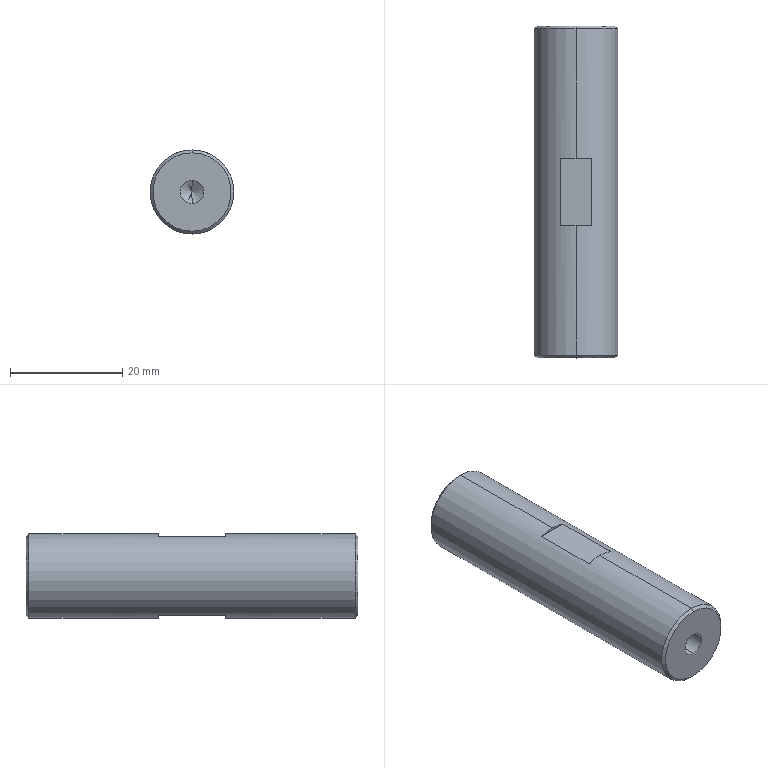Part | STEP file | ND25021-01-JDKM-72-TL | 1 solid | 22 faces | box 15 x 59.2 x 15 mm | volume 10051 mm3 | cone 8 | plane 8 | cylinder 6 | commonest cylinder face diameters 4.2 x4 15 x2
STEP:
#1=CARTESIAN_POINT('',(0.,0.,0.));
#2=DIRECTION('',(0.,0.,1.));
#3=DIRECTION('',(1.,0.,0.));
#4=AXIS2_PLACEMENT_3D('',#1,#2,#3);
#5=CARTESIAN_POINT('',(0.,29.6,7.));
#6=VERTEX_POINT('',#5);
#7=CARTESIAN_POINT('',(0.,29.6,-7.));
#8=VERTEX_POINT('',#7);
#9=CARTESIAN_POINT('',(0.,29.6,0.));
#10=DIRECTION('',(0.,1.,0.));
#11=DIRECTION('',(0.,0.,1.));
#12=AXIS2_PLACEMENT_3D('',#9,#10,#11);
#13=CIRCLE('',#12,7.);
#14=CARTESIAN_POINT('',(0.,29.6,0.));
#15=DIRECTION('',(0.,-1.,0.));
#16=DIRECTION('',(0.,0.,-1.));
#17=AXIS2_PLACEMENT_3D('',#14,#15,#16);
#18=CONICAL_SURFACE('',#17,7.,0.7854);
#19=CARTESIAN_POINT('',(3.142,0.));
#20=DIRECTION('',(-1.,0.));
#21=VECTOR('',#20,1.);
#22=LINE('',#19,#21);
#23=(GEOMETRIC_REPRESENTATION_CONTEXT(2)PARAMETRIC_REPRESENTATION_CONTEXT()REPRESENTATION_CONTEXT('',''));
#24=DEFINITIONAL_REPRESENTATION('',(#22),#23);
#25=PCURVE('',#18,#24);
#26=CARTESIAN_POINT('',(0.,29.6,0.));
#27=DIRECTION('',(0.,1.,0.));
#28=DIRECTION('',(0.,0.,1.));
#29=AXIS2_PLACEMENT_3D('',#26,#27,#28);
#30=PLANE('',#29);
#31=CARTESIAN_POINT('',(0.,0.));
#32=DIRECTION('',(1.,0.));
#33=AXIS2_PLACEMENT_2D('',#31,#32);
#34=CIRCLE('',#33,7.);
#35=(GEOMETRIC_REPRESENTATION_CONTEXT(2)PARAMETRIC_REPRESENTATION_CONTEXT()REPRESENTATION_CONTEXT('',''));
#36=DEFINITIONAL_REPRESENTATION('',(#34),#35);
#37=PCURVE('',#30,#36);
#38=SURFACE_CURVE('',#13,(#25,#37),.PCURVE_S1.);
#39=EDGE_CURVE('',#6,#8,#38,.T.);
#40=ORIENTED_EDGE('',*,*,#39,.F.);
#41=CARTESIAN_POINT('',(0.,29.1,7.5));
#42=VERTEX_POINT('',#41);
#43=CARTESIAN_POINT('',(0.,29.6,7.));
#44=DIRECTION('',(0.,-0.7071,0.7071));
#45=VECTOR('',#44,1.);
#46=LINE('',#43,#45);
#47=CARTESIAN_POINT('',(3.142,0.));
#48=DIRECTION('',(0.,1.));
#49=VECTOR('',#48,1.);
#50=LINE('',#47,#49);
#51=(GEOMETRIC_REPRESENTATION_CONTEXT(2)PARAMETRIC_REPRESENTATION_CONTEXT()REPRESENTATION_CONTEXT('',''));
#52=DEFINITIONAL_REPRESENTATION('',(#50),#51);
#53=PCURVE('',#18,#52);
#54=CARTESIAN_POINT('',(0.,29.6,0.));
#55=DIRECTION('',(0.,-1.,0.));
#56=DIRECTION('',(0.,0.,-1.));
#57=AXIS2_PLACEMENT_3D('',#54,#55,#56);
#58=CONICAL_SURFACE('',#57,7.,0.7854);
#59=CARTESIAN_POINT('',(3.142,0.));
#60=DIRECTION('',(0.,1.));
#61=VECTOR('',#60,1.);
#62=LINE('',#59,#61);
#63=(GEOMETRIC_REPRESENTATION_CONTEXT(2)PARAMETRIC_REPRESENTATION_CONTEXT()REPRESENTATION_CONTEXT('',''));
#64=DEFINITIONAL_REPRESENTATION('',(#62),#63);
#65=PCURVE('',#58,#64);
#66=SURFACE_CURVE('',#46,(#53,#65),.PCURVE_S1.);
#67=EDGE_CURVE('',#6,#42,#66,.T.);
#68=ORIENTED_EDGE('',*,*,#67,.T.);
#69=CARTESIAN_POINT('',(0.,29.1,-7.5));
#70=VERTEX_POINT('',#69);
#71=CARTESIAN_POINT('',(0.,29.1,0.));
#72=DIRECTION('',(0.,-1.,0.));
#73=DIRECTION('',(0.,0.,1.));
#74=AXIS2_PLACEMENT_3D('',#71,#72,#73);
#75=CIRCLE('',#74,7.5);
#76=CARTESIAN_POINT('',(-3.142,0.5));
#77=DIRECTION('',(1.,0.));
#78=VECTOR('',#77,1.);
#79=LINE('',#76,#78);
#80=(GEOMETRIC_REPRESENTATION_CONTEXT(2)PARAMETRIC_REPRESENTATION_CONTEXT()REPRESENTATION_CONTEXT('',''));
#81=DEFINITIONAL_REPRESENTATION('',(#79),#80);
#82=PCURVE('',#18,#81);
#83=CARTESIAN_POINT('',(0.,29.6,0.));
#84=DIRECTION('',(0.,-1.,0.));
#85=DIRECTION('',(0.,0.,-1.));
#86=AXIS2_PLACEMENT_3D('',#83,#84,#85);
#87=CYLINDRICAL_SURFACE('',#86,7.5);
#88=CARTESIAN_POINT('',(-3.142,0.5));
#89=DIRECTION('',(1.,0.));
#90=VECTOR('',#89,1.);
#91=LINE('',#88,#90);
#92=(GEOMETRIC_REPRESENTATION_CONTEXT(2)PARAMETRIC_REPRESENTATION_CONTEXT()REPRESENTATION_CONTEXT('',''));
#93=DEFINITIONAL_REPRESENTATION('',(#91),#92);
#94=PCURVE('',#87,#93);
#95=SURFACE_CURVE('',#75,(#82,#94),.PCURVE_S1.);
#96=EDGE_CURVE('',#70,#42,#95,.T.);
#97=ORIENTED_EDGE('',*,*,#96,.F.);
#98=CARTESIAN_POINT('',(0.,29.6,-7.));
#99=DIRECTION('',(0.,-0.7071,-0.7071));
#100=VECTOR('',#99,1.);
#101=LINE('',#98,#100);
#102=CARTESIAN_POINT('',(0.,0.));
#103=DIRECTION('',(0.,1.));
#104=VECTOR('',#103,1.);
#105=LINE('',#102,#104);
#106=(GEOMETRIC_REPRESENTATION_CONTEXT(2)PARAMETRIC_REPRESENTATION_CONTEXT()REPRESENTATION_CONTEXT('',''));
#107=DEFINITIONAL_REPRESENTATION('',(#105),#106);
#108=PCURVE('',#18,#107);
#109=CARTESIAN_POINT('',(6.283,0.));
#110=DIRECTION('',(0.,1.));
#111=VECTOR('',#110,1.);
#112=LINE('',#109,#111);
#113=(GEOMETRIC_REPRESENTATION_CONTEXT(2)PARAMETRIC_REPRESENTATION_CONTEXT()REPRESENTATION_CONTEXT('',''));
#114=DEFINITIONAL_REPRESENTATION('',(#112),#113);
#115=PCURVE('',#58,#114);
#116=SURFACE_CURVE('',#101,(#108,#115),.PCURVE_S1.);
#117=EDGE_CURVE('',#8,#70,#116,.T.);
#118=ORIENTED_EDGE('',*,*,#117,.F.);
#119=EDGE_LOOP('',(#40,#68,#97,#118));
#120=FACE_BOUND('',#119,.T.);
#121=ADVANCED_FACE('',(#120),#18,.T.);
#122=CARTESIAN_POINT('',(0.,-29.6,-7.));
#123=VERTEX_POINT('',#122);
#124=CARTESIAN_POINT('',(0.,-29.6,7.));
#125=VERTEX_POINT('',#124);
#126=CARTESIAN_POINT('',(0.,-29.6,0.));
#127=DIRECTION('',(0.,-1.,0.));
#128=DIRECTION('',(0.,0.,1.));
#129=AXIS2_PLACEMENT_3D('',#126,#127,#128);
#130=CIRCLE('',#129,7.);
#131=CARTESIAN_POINT('',(0.,-29.1,0.));
#132=DIRECTION('',(0.,1.,0.));
#133=DIRECTION('',(0.,0.,1.));
#134=AXIS2_PLACEMENT_3D('',#131,#132,#133);
#135=CONICAL_SURFACE('',#134,7.5,0.7854);
#136=CARTESIAN_POINT('',(6.283,-0.5));
#137=DIRECTION('',(-1.,0.));
#138=VECTOR('',#137,1.);
#139=LINE('',#136,#138);
#140=(GEOMETRIC_REPRESENTATION_CONTEXT(2)PARAMETRIC_REPRESENTATION_CONTEXT()REPRESENTATION_CONTEXT('',''));
#141=DEFINITIONAL_REPRESENTATION('',(#139),#140);
#142=PCURVE('',#135,#141);
#143=CARTESIAN_POINT('',(0.,-29.6,0.));
#144=DIRECTION('',(0.,1.,0.));
#145=DIRECTION('',(0.,0.,1.));
#146=AXIS2_PLACEMENT_3D('',#143,#144,#145);
#147=PLANE('',#146);
#148=CARTESIAN_POINT('',(7.,0.));
#149=CARTESIAN_POINT('',(7.,-12.124));
#150=CARTESIAN_POINT('',(-3.5,-6.062));
#151=CARTESIAN_POINT('',(-14.,0.));
#152=CARTESIAN_POINT('',(-3.5,6.062));
#153=CARTESIAN_POINT('',(7.,12.124));
#154=CARTESIAN_POINT('',(7.,0.));
#155=(BOUNDED_CURVE()B_SPLINE_CURVE(2,(#148,#149,#150,#151,#152,#153,#154),.UNSPECIFIED.,.T.,.F.)B_SPLINE_CURVE_WITH_KNOTS((1,2,2,2,2,1),(-2.094,0.,2.094,4.189,6.283,8.378),.UNSPECIFIED.)CURVE()GEOMETRIC_REPRESENTATION_ITEM()RATIONAL_B_SPLINE_CURVE((1.,0.5,1.,0.5,1.,0.5,1.))REPRESENTATION_ITEM(''));
#156=(GEOMETRIC_REPRESENTATION_CONTEXT(2)PARAMETRIC_REPRESENTATION_CONTEXT()REPRESENTATION_CONTEXT('',''));
#157=DEFINITIONAL_REPRESENTATION('',(#155),#156);
#158=PCURVE('',#147,#157);
#159=SURFACE_CURVE('',#130,(#142,#158),.PCURVE_S1.);
#160=EDGE_CURVE('',#123,#125,#159,.T.);
#161=ORIENTED_EDGE('',*,*,#160,.F.);
#162=CARTESIAN_POINT('',(0.,-29.1,-7.5));
#163=VERTEX_POINT('',#162);
#164=CARTESIAN_POINT('',(0.,-29.1,-7.5));
#165=DIRECTION('',(0.,0.7071,-0.7071));
#166=VECTOR('',#165,1.);
#167=LINE('',#164,#166);
#168=CARTESIAN_POINT('',(3.142,0.));
#169=DIRECTION('',(0.,1.));
#170=VECTOR('',#169,1.);
#171=LINE('',#168,#170);
#172=(GEOMETRIC_REPRESENTATION_CONTEXT(2)PARAMETRIC_REPRESENTATION_CONTEXT()REPRESENTATION_CONTEXT('',''));
#173=DEFINITIONAL_REPRESENTATION('',(#171),#172);
#174=PCURVE('',#135,#173);
#175=CARTESIAN_POINT('',(0.,-29.1,0.));
#176=DIRECTION('',(0.,1.,0.));
#177=DIRECTION('',(0.,0.,1.));
#178=AXIS2_PLACEMENT_3D('',#175,#176,#177);
#179=CONICAL_SURFACE('',#178,7.5,0.7854);
#180=CARTESIAN_POINT('',(3.142,0.));
#181=DIRECTION('',(0.,1.));
#182=VECTOR('',#181,1.);
#183=LINE('',#180,#182);
#184=(GEOMETRIC_REPRESENTATION_CONTEXT(2)PARAMETRIC_REPRESENTATION_CONTEXT()REPRESENTATION_CONTEXT('',''));
#185=DEFINITIONAL_REPRESENTATION('',(#183),#184);
#186=PCURVE('',#179,#185);
#187=SURFACE_CURVE('',#167,(#174,#186),.PCURVE_S1.);
#188=EDGE_CURVE('',#123,#163,#187,.T.);
#189=ORIENTED_EDGE('',*,*,#188,.T.);
#190=CARTESIAN_POINT('',(0.,-29.1,7.5));
#191=VERTEX_POINT('',#190);
#192=CARTESIAN_POINT('',(0.,-29.1,0.));
#193=DIRECTION('',(0.,1.,0.));
#194=DIRECTION('',(0.,0.,1.));
#195=AXIS2_PLACEMENT_3D('',#192,#193,#194);
#196=CIRCLE('',#195,7.5);
#197=CARTESIAN_POINT('',(0.,0.));
#198=DIRECTION('',(1.,0.));
#199=VECTOR('',#198,1.);
#200=LINE('',#197,#199);
#201=(GEOMETRIC_REPRESENTATION_CONTEXT(2)PARAMETRIC_REPRESENTATION_CONTEXT()REPRESENTATION_CONTEXT('',''));
#202=DEFINITIONAL_REPRESENTATION('',(#200),#201);
#203=PCURVE('',#135,#202);
#204=CARTESIAN_POINT('',(3.142,58.7));
#205=DIRECTION('',(-1.,0.));
#206=VECTOR('',#205,1.);
#207=LINE('',#204,#206);
#208=(GEOMETRIC_REPRESENTATION_CONTEXT(2)PARAMETRIC_REPRESENTATION_CONTEXT()REPRESENTATION_CONTEXT('',''));
#209=DEFINITIONAL_REPRESENTATION('',(#207),#208);
#210=PCURVE('',#87,#209);
#211=SURFACE_CURVE('',#196,(#203,#210),.PCURVE_S1.);
#212=EDGE_CURVE('',#191,#163,#211,.T.);
#213=ORIENTED_EDGE('',*,*,#212,.F.);
#214=CARTESIAN_POINT('',(0.,-29.1,7.5));
#215=DIRECTION('',(0.,0.7071,0.7071));
#216=VECTOR('',#215,1.);
#217=LINE('',#214,#216);
#218=CARTESIAN_POINT('',(0.,0.));
#219=DIRECTION('',(0.,1.));
#220=VECTOR('',#219,1.);
#221=LINE('',#218,#220);
#222=(GEOMETRIC_REPRESENTATION_CONTEXT(2)PARAMETRIC_REPRESENTATION_CONTEXT()REPRESENTATION_CONTEXT('',''));
#223=DEFINITIONAL_REPRESENTATION('',(#221),#222);
#224=PCURVE('',#135,#223);
#225=CARTESIAN_POINT('',(6.283,0.));
#226=DIRECTION('',(0.,1.));
#227=VECTOR('',#226,1.);
#228=LINE('',#225,#227);
#229=(GEOMETRIC_REPRESENTATION_CONTEXT(2)PARAMETRIC_REPRESENTATION_CONTEXT()REPRESENTATION_CONTEXT('',''));
#230=DEFINITIONAL_REPRESENTATION('',(#228),#229);
#231=PCURVE('',#179,#230);
#232=SURFACE_CURVE('',#217,(#224,#231),.PCURVE_S1.);
#233=EDGE_CURVE('',#125,#191,#232,.T.);
#234=ORIENTED_EDGE('',*,*,#233,.F.);
#235=EDGE_LOOP('',(#161,#189,#213,#234));
#236=FACE_BOUND('',#235,.T.);
#237=ADVANCED_FACE('',(#236),#135,.T.);
#238=CARTESIAN_POINT('',(0.,-17.2,-2.1));
#239=VERTEX_POINT('',#238);
#240=CARTESIAN_POINT('',(0.,-29.6,-2.1));
#241=VERTEX_POINT('',#240);
#242=CARTESIAN_POINT('',(0.,-29.6,-2.1));
#243=DIRECTION('',(0.,-1.,0.));
#244=VECTOR('',#243,1.);
#245=LINE('',#242,#244);
#246=CARTESIAN_POINT('',(0.,-29.6,0.));
#247=DIRECTION('',(0.,-1.,0.));
#248=DIRECTION('',(0.,0.,-1.));
#249=AXIS2_PLACEMENT_3D('',#246,#247,#248);
#250=CYLINDRICAL_SURFACE('',#249,2.1);
#251=CARTESIAN_POINT('',(6.283,0.));
#252=DIRECTION('',(0.,1.));
#253=VECTOR('',#252,1.);
#254=LINE('',#251,#253);
#255=(GEOMETRIC_REPRESENTATION_CONTEXT(2)PARAMETRIC_REPRESENTATION_CONTEXT()REPRESENTATION_CONTEXT('',''));
#256=DEFINITIONAL_REPRESENTATION('',(#254),#255);
#257=PCURVE('',#250,#256);
#258=CARTESIAN_POINT('',(0.,-29.6,0.));
#259=DIRECTION('',(0.,-1.,0.));
#260=DIRECTION('',(0.,0.,-1.));
#261=AXIS2_PLACEMENT_3D('',#258,#259,#260);
#262=CYLINDRICAL_SURFACE('',#261,2.1);
#263=CARTESIAN_POINT('',(0.,0.));
#264=DIRECTION('',(0.,1.));
#265=VECTOR('',#264,1.);
#266=LINE('',#263,#265);
#267=(GEOMETRIC_REPRESENTATION_CONTEXT(2)PARAMETRIC_REPRESENTATION_CONTEXT()REPRESENTATION_CONTEXT('',''));
#268=DEFINITIONAL_REPRESENTATION('',(#266),#267);
#269=PCURVE('',#262,#268);
#270=SURFACE_CURVE('',#245,(#257,#269),.PCURVE_S1.);
#271=EDGE_CURVE('',#239,#241,#270,.T.);
#272=ORIENTED_EDGE('',*,*,#271,.T.);
#273=CARTESIAN_POINT('',(0.,-29.6,2.1));
#274=VERTEX_POINT('',#273);
#275=CARTESIAN_POINT('',(0.,-29.6,0.));
#276=DIRECTION('',(0.,-1.,0.));
#277=DIRECTION('',(0.,0.,-1.));
#278=AXIS2_PLACEMENT_3D('',#275,#276,#277);
#279=CIRCLE('',#278,2.1);
#280=CARTESIAN_POINT('',(0.,0.));
#281=DIRECTION('',(1.,0.));
#282=VECTOR('',#281,1.);
#283=LINE('',#280,#282);
#284=(GEOMETRIC_REPRESENTATION_CONTEXT(2)PARAMETRIC_REPRESENTATION_CONTEXT()REPRESENTATION_CONTEXT('',''));
#285=DEFINITIONAL_REPRESENTATION('',(#283),#284);
#286=PCURVE('',#250,#285);
#287=CARTESIAN_POINT('',(-2.1,0.));
#288=CARTESIAN_POINT('',(-2.1,3.637));
#289=CARTESIAN_POINT('',(1.05,1.819));
#290=CARTESIAN_POINT('',(4.2,0.));
#291=CARTESIAN_POINT('',(1.05,-1.819));
#292=CARTESIAN_POINT('',(-2.1,-3.637));
#293=CARTESIAN_POINT('',(-2.1,0.));
#294=(BOUNDED_CURVE()B_SPLINE_CURVE(2,(#287,#288,#289,#290,#291,#292,#293),.UNSPECIFIED.,.T.,.F.)B_SPLINE_CURVE_WITH_KNOTS((1,2,2,2,2,1),(-2.094,0.,2.094,4.189,6.283,8.378),.UNSPECIFIED.)CURVE()GEOMETRIC_REPRESENTATION_ITEM()RATIONAL_B_SPLINE_CURVE((1.,0.5,1.,0.5,1.,0.5,1.))REPRESENTATION_ITEM(''));
#295=(GEOMETRIC_REPRESENTATION_CONTEXT(2)PARAMETRIC_REPRESENTATION_CONTEXT()REPRESENTATION_CONTEXT('',''));
#296=DEFINITIONAL_REPRESENTATION('',(#294),#295);
#297=PCURVE('',#147,#296);
#298=SURFACE_CURVE('',#279,(#286,#297),.PCURVE_S1.);
#299=EDGE_CURVE('',#274,#241,#298,.T.);
#300=ORIENTED_EDGE('',*,*,#299,.F.);
#301=CARTESIAN_POINT('',(0.,-17.2,2.1));
#302=VERTEX_POINT('',#301);
#303=CARTESIAN_POINT('',(0.,-29.6,2.1));
#304=DIRECTION('',(0.,-1.,0.));
#305=VECTOR('',#304,1.);
#306=LINE('',#303,#305);
#307=CARTESIAN_POINT('',(3.142,0.));
#308=DIRECTION('',(0.,1.));
#309=VECTOR('',#308,1.);
#310=LINE('',#307,#309);
#311=(GEOMETRIC_REPRESENTATION_CONTEXT(2)PARAMETRIC_REPRESENTATION_CONTEXT()REPRESENTATION_CONTEXT('',''));
#312=DEFINITIONAL_REPRESENTATION('',(#310),#311);
#313=PCURVE('',#250,#312);
#314=CARTESIAN_POINT('',(3.142,0.));
#315=DIRECTION('',(0.,1.));
#316=VECTOR('',#315,1.);
#317=LINE('',#314,#316);
#318=(GEOMETRIC_REPRESENTATION_CONTEXT(2)PARAMETRIC_REPRESENTATION_CONTEXT()REPRESENTATION_CONTEXT('',''));
#319=DEFINITIONAL_REPRESENTATION('',(#317),#318);
#320=PCURVE('',#262,#319);
#321=SURFACE_CURVE('',#306,(#313,#320),.PCURVE_S1.);
#322=EDGE_CURVE('',#302,#274,#321,.T.);
#323=ORIENTED_EDGE('',*,*,#322,.F.);
#324=CARTESIAN_POINT('',(0.,-17.2,0.));
#325=DIRECTION('',(0.,-1.,0.));
#326=DIRECTION('',(0.,0.,-1.));
#327=AXIS2_PLACEMENT_3D('',#324,#325,#326);
#328=CIRCLE('',#327,2.1);
#329=CARTESIAN_POINT('',(0.,-12.4));
#330=DIRECTION('',(1.,0.));
#331=VECTOR('',#330,1.);
#332=LINE('',#329,#331);
#333=(GEOMETRIC_REPRESENTATION_CONTEXT(2)PARAMETRIC_REPRESENTATION_CONTEXT()REPRESENTATION_CONTEXT('',''));
#334=DEFINITIONAL_REPRESENTATION('',(#332),#333);
#335=PCURVE('',#250,#334);
#336=CARTESIAN_POINT('',(0.,-17.2,0.));
#337=DIRECTION('',(0.,-1.,0.));
#338=DIRECTION('',(0.,0.,-1.));
#339=AXIS2_PLACEMENT_3D('',#336,#337,#338);
#340=CONICAL_SURFACE('',#339,2.1,1.03);
#341=CARTESIAN_POINT('',(0.,0.));
#342=DIRECTION('',(1.,0.));
#343=VECTOR('',#342,1.);
#344=LINE('',#341,#343);
#345=(GEOMETRIC_REPRESENTATION_CONTEXT(2)PARAMETRIC_REPRESENTATION_CONTEXT()REPRESENTATION_CONTEXT('',''));
#346=DEFINITIONAL_REPRESENTATION('',(#344),#345);
#347=PCURVE('',#340,#346);
#348=SURFACE_CURVE('',#328,(#335,#347),.PCURVE_S1.);
#349=EDGE_CURVE('',#302,#239,#348,.T.);
#350=ORIENTED_EDGE('',*,*,#349,.T.);
#351=EDGE_LOOP('',(#272,#300,#323,#350));
#352=FACE_BOUND('',#351,.F.);
#353=ADVANCED_FACE('',(#352),#250,.F.);
#354=ORIENTED_EDGE('',*,*,#349,.F.);
#355=CARTESIAN_POINT('',(0.,-15.938,0.));
#356=VERTEX_POINT('',#355);
#357=CARTESIAN_POINT('',(0.,-17.2,2.1));
#358=DIRECTION('',(0.,-0.515,0.8572));
#359=VECTOR('',#358,1.);
#360=LINE('',#357,#359);
#361=CARTESIAN_POINT('',(3.142,0.));
#362=DIRECTION('',(0.,1.));
#363=VECTOR('',#362,1.);
#364=LINE('',#361,#363);
#365=(GEOMETRIC_REPRESENTATION_CONTEXT(2)PARAMETRIC_REPRESENTATION_CONTEXT()REPRESENTATION_CONTEXT('',''));
#366=DEFINITIONAL_REPRESENTATION('',(#364),#365);
#367=PCURVE('',#340,#366);
#368=CARTESIAN_POINT('',(0.,-17.2,0.));
#369=DIRECTION('',(0.,-1.,0.));
#370=DIRECTION('',(0.,0.,-1.));
#371=AXIS2_PLACEMENT_3D('',#368,#369,#370);
#372=CONICAL_SURFACE('',#371,2.1,1.03);
#373=CARTESIAN_POINT('',(3.142,0.));
#374=DIRECTION('',(0.,1.));
#375=VECTOR('',#374,1.);
#376=LINE('',#373,#375);
#377=(GEOMETRIC_REPRESENTATION_CONTEXT(2)PARAMETRIC_REPRESENTATION_CONTEXT()REPRESENTATION_CONTEXT('',''));
#378=DEFINITIONAL_REPRESENTATION('',(#376),#377);
#379=PCURVE('',#372,#378);
#380=SURFACE_CURVE('',#360,(#367,#379),.PCURVE_S1.);
#381=EDGE_CURVE('',#356,#302,#380,.T.);
#382=ORIENTED_EDGE('',*,*,#381,.F.);
#383=CARTESIAN_POINT('',(0.,-17.2,-2.1));
#384=DIRECTION('',(0.,-0.515,-0.8572));
#385=VECTOR('',#384,1.);
#386=LINE('',#383,#385);
#387=CARTESIAN_POINT('',(6.283,0.));
#388=DIRECTION('',(0.,1.));
#389=VECTOR('',#388,1.);
#390=LINE('',#387,#389);
#391=(GEOMETRIC_REPRESENTATION_CONTEXT(2)PARAMETRIC_REPRESENTATION_CONTEXT()REPRESENTATION_CONTEXT('',''));
#392=DEFINITIONAL_REPRESENTATION('',(#390),#391);
#393=PCURVE('',#340,#392);
#394=CARTESIAN_POINT('',(0.,0.));
#395=DIRECTION('',(0.,1.));
#396=VECTOR('',#395,1.);
#397=LINE('',#394,#396);
#398=(GEOMETRIC_REPRESENTATION_CONTEXT(2)PARAMETRIC_REPRESENTATION_CONTEXT()REPRESENTATION_CONTEXT('',''));
#399=DEFINITIONAL_REPRESENTATION('',(#397),#398);
#400=PCURVE('',#372,#399);
#401=SURFACE_CURVE('',#386,(#393,#400),.PCURVE_S1.);
#402=EDGE_CURVE('',#356,#239,#401,.T.);
#403=ORIENTED_EDGE('',*,*,#402,.T.);
#404=EDGE_LOOP('',(#354,#382,#403));
#405=FACE_BOUND('',#404,.F.);
#406=ADVANCED_FACE('',(#405),#340,.F.);
#407=CARTESIAN_POINT('',(0.,17.2,2.1));
#408=VERTEX_POINT('',#407);
#409=CARTESIAN_POINT('',(0.,29.6,2.1));
#410=VERTEX_POINT('',#409);
#411=CARTESIAN_POINT('',(0.,29.6,2.1));
#412=DIRECTION('',(0.,1.,0.));
#413=VECTOR('',#412,1.);
#414=LINE('',#411,#413);
#415=CARTESIAN_POINT('',(0.,29.6,0.));
#416=DIRECTION('',(0.,1.,0.));
#417=DIRECTION('',(0.,0.,1.));
#418=AXIS2_PLACEMENT_3D('',#415,#416,#417);
#419=CYLINDRICAL_SURFACE('',#418,2.1);
#420=CARTESIAN_POINT('',(6.283,0.));
#421=DIRECTION('',(0.,1.));
#422=VECTOR('',#421,1.);
#423=LINE('',#420,#422);
#424=(GEOMETRIC_REPRESENTATION_CONTEXT(2)PARAMETRIC_REPRESENTATION_CONTEXT()REPRESENTATION_CONTEXT('',''));
#425=DEFINITIONAL_REPRESENTATION('',(#423),#424);
#426=PCURVE('',#419,#425);
#427=CARTESIAN_POINT('',(0.,29.6,0.));
#428=DIRECTION('',(0.,1.,0.));
#429=DIRECTION('',(0.,0.,1.));
#430=AXIS2_PLACEMENT_3D('',#427,#428,#429);
#431=CYLINDRICAL_SURFACE('',#430,2.1);
#432=CARTESIAN_POINT('',(0.,0.));
#433=DIRECTION('',(0.,1.));
#434=VECTOR('',#433,1.);
#435=LINE('',#432,#434);
#436=(GEOMETRIC_REPRESENTATION_CONTEXT(2)PARAMETRIC_REPRESENTATION_CONTEXT()REPRESENTATION_CONTEXT('',''));
#437=DEFINITIONAL_REPRESENTATION('',(#435),#436);
#438=PCURVE('',#431,#437);
#439=SURFACE_CURVE('',#414,(#426,#438),.PCURVE_S1.);
#440=EDGE_CURVE('',#408,#410,#439,.T.);
#441=ORIENTED_EDGE('',*,*,#440,.T.);
#442=CARTESIAN_POINT('',(0.,29.6,-2.1));
#443=VERTEX_POINT('',#442);
#444=CARTESIAN_POINT('',(0.,29.6,0.));
#445=DIRECTION('',(0.,1.,0.));
#446=DIRECTION('',(0.,0.,1.));
#447=AXIS2_PLACEMENT_3D('',#444,#445,#446);
#448=CIRCLE('',#447,2.1);
#449=CARTESIAN_POINT('',(0.,0.));
#450=DIRECTION('',(1.,0.));
#451=VECTOR('',#450,1.);
#452=LINE('',#449,#451);
#453=(GEOMETRIC_REPRESENTATION_CONTEXT(2)PARAMETRIC_REPRESENTATION_CONTEXT()REPRESENTATION_CONTEXT('',''));
#454=DEFINITIONAL_REPRESENTATION('',(#452),#453);
#455=PCURVE('',#419,#454);
#456=CARTESIAN_POINT('',(0.,0.));
#457=DIRECTION('',(1.,0.));
#458=AXIS2_PLACEMENT_2D('',#456,#457);
#459=CIRCLE('',#458,2.1);
#460=(GEOMETRIC_REPRESENTATION_CONTEXT(2)PARAMETRIC_REPRESENTATION_CONTEXT()REPRESENTATION_CONTEXT('',''));
#461=DEFINITIONAL_REPRESENTATION('',(#459),#460);
#462=PCURVE('',#30,#461);
#463=SURFACE_CURVE('',#448,(#455,#462),.PCURVE_S1.);
#464=EDGE_CURVE('',#443,#410,#463,.T.);
#465=ORIENTED_EDGE('',*,*,#464,.F.);
#466=CARTESIAN_POINT('',(0.,17.2,-2.1));
#467=VERTEX_POINT('',#466);
#468=CARTESIAN_POINT('',(0.,29.6,-2.1));
#469=DIRECTION('',(0.,1.,0.));
#470=VECTOR('',#469,1.);
#471=LINE('',#468,#470);
#472=CARTESIAN_POINT('',(3.142,0.));
#473=DIRECTION('',(0.,1.));
#474=VECTOR('',#473,1.);
#475=LINE('',#472,#474);
#476=(GEOMETRIC_REPRESENTATION_CONTEXT(2)PARAMETRIC_REPRESENTATION_CONTEXT()REPRESENTATION_CONTEXT('',''));
#477=DEFINITIONAL_REPRESENTATION('',(#475),#476);
#478=PCURVE('',#419,#477);
#479=CARTESIAN_POINT('',(3.142,0.));
#480=DIRECTION('',(0.,1.));
#481=VECTOR('',#480,1.);
#482=LINE('',#479,#481);
#483=(GEOMETRIC_REPRESENTATION_CONTEXT(2)PARAMETRIC_REPRESENTATION_CONTEXT()REPRESENTATION_CONTEXT('',''));
#484=DEFINITIONAL_REPRESENTATION('',(#482),#483);
#485=PCURVE('',#431,#484);
#486=SURFACE_CURVE('',#471,(#478,#485),.PCURVE_S1.);
#487=EDGE_CURVE('',#467,#443,#486,.T.);
#488=ORIENTED_EDGE('',*,*,#487,.F.);
#489=CARTESIAN_POINT('',(0.,17.2,0.));
#490=DIRECTION('',(0.,1.,0.));
#491=DIRECTION('',(0.,0.,1.));
#492=AXIS2_PLACEMENT_3D('',#489,#490,#491);
#493=CIRCLE('',#492,2.1);
#494=CARTESIAN_POINT('',(0.,-12.4));
#495=DIRECTION('',(1.,0.));
#496=VECTOR('',#495,1.);
#497=LINE('',#494,#496);
#498=(GEOMETRIC_REPRESENTATION_CONTEXT(2)PARAMETRIC_REPRESENTATION_CONTEXT()REPRESENTATION_CONTEXT('',''));
#499=DEFINITIONAL_REPRESENTATION('',(#497),#498);
#500=PCURVE('',#419,#499);
#501=CARTESIAN_POINT('',(0.,17.2,0.));
#502=DIRECTION('',(0.,1.,0.));
#503=DIRECTION('',(0.,0.,1.));
#504=AXIS2_PLACEMENT_3D('',#501,#502,#503);
#505=CONICAL_SURFACE('',#504,2.1,1.03);
#506=CARTESIAN_POINT('',(0.,0.));
#507=DIRECTION('',(1.,0.));
#508=VECTOR('',#507,1.);
#509=LINE('',#506,#508);
#510=(GEOMETRIC_REPRESENTATION_CONTEXT(2)PARAMETRIC_REPRESENTATION_CONTEXT()REPRESENTATION_CONTEXT('',''));
#511=DEFINITIONAL_REPRESENTATION('',(#509),#510);
#512=PCURVE('',#505,#511);
#513=SURFACE_CURVE('',#493,(#500,#512),.PCURVE_S1.);
#514=EDGE_CURVE('',#467,#408,#513,.T.);
#515=ORIENTED_EDGE('',*,*,#514,.T.);
#516=EDGE_LOOP('',(#441,#465,#488,#515));
#517=FACE_BOUND('',#516,.F.);
#518=ADVANCED_FACE('',(#517),#419,.F.);
#519=ORIENTED_EDGE('',*,*,#514,.F.);
#520=CARTESIAN_POINT('',(0.,15.938,0.));
#521=VERTEX_POINT('',#520);
#522=CARTESIAN_POINT('',(0.,17.2,-2.1));
#523=DIRECTION('',(0.,0.515,-0.8572));
#524=VECTOR('',#523,1.);
#525=LINE('',#522,#524);
#526=CARTESIAN_POINT('',(3.142,0.));
#527=DIRECTION('',(0.,1.));
#528=VECTOR('',#527,1.);
#529=LINE('',#526,#528);
#530=(GEOMETRIC_REPRESENTATION_CONTEXT(2)PARAMETRIC_REPRESENTATION_CONTEXT()REPRESENTATION_CONTEXT('',''));
#531=DEFINITIONAL_REPRESENTATION('',(#529),#530);
#532=PCURVE('',#505,#531);
#533=CARTESIAN_POINT('',(0.,17.2,0.));
#534=DIRECTION('',(0.,1.,0.));
#535=DIRECTION('',(0.,0.,1.));
#536=AXIS2_PLACEMENT_3D('',#533,#534,#535);
#537=CONICAL_SURFACE('',#536,2.1,1.03);
#538=CARTESIAN_POINT('',(3.142,0.));
#539=DIRECTION('',(0.,1.));
#540=VECTOR('',#539,1.);
#541=LINE('',#538,#540);
#542=(GEOMETRIC_REPRESENTATION_CONTEXT(2)PARAMETRIC_REPRESENTATION_CONTEXT()REPRESENTATION_CONTEXT('',''));
#543=DEFINITIONAL_REPRESENTATION('',(#541),#542);
#544=PCURVE('',#537,#543);
#545=SURFACE_CURVE('',#525,(#532,#544),.PCURVE_S1.);
#546=EDGE_CURVE('',#521,#467,#545,.T.);
#547=ORIENTED_EDGE('',*,*,#546,.F.);
#548=CARTESIAN_POINT('',(0.,17.2,2.1));
#549=DIRECTION('',(0.,0.515,0.8572));
#550=VECTOR('',#549,1.);
#551=LINE('',#548,#550);
#552=CARTESIAN_POINT('',(6.283,0.));
#553=DIRECTION('',(0.,1.));
#554=VECTOR('',#553,1.);
#555=LINE('',#552,#554);
#556=(GEOMETRIC_REPRESENTATION_CONTEXT(2)PARAMETRIC_REPRESENTATION_CONTEXT()REPRESENTATION_CONTEXT('',''));
#557=DEFINITIONAL_REPRESENTATION('',(#555),#556);
#558=PCURVE('',#505,#557);
#559=CARTESIAN_POINT('',(0.,0.));
#560=DIRECTION('',(0.,1.));
#561=VECTOR('',#560,1.);
#562=LINE('',#559,#561);
#563=(GEOMETRIC_REPRESENTATION_CONTEXT(2)PARAMETRIC_REPRESENTATION_CONTEXT()REPRESENTATION_CONTEXT('',''));
#564=DEFINITIONAL_REPRESENTATION('',(#562),#563);
#565=PCURVE('',#537,#564);
#566=SURFACE_CURVE('',#551,(#558,#565),.PCURVE_S1.);
#567=EDGE_CURVE('',#521,#408,#566,.T.);
#568=ORIENTED_EDGE('',*,*,#567,.T.);
#569=EDGE_LOOP('',(#519,#547,#568));
#570=FACE_BOUND('',#569,.F.);
#571=ADVANCED_FACE('',(#570),#505,.F.);
#572=ORIENTED_EDGE('',*,*,#96,.T.);
#573=CARTESIAN_POINT('',(0.,6.,7.5));
#574=VERTEX_POINT('',#573);
#575=CARTESIAN_POINT('',(0.,29.6,7.5));
#576=DIRECTION('',(0.,-1.,0.));
#577=VECTOR('',#576,1.);
#578=LINE('',#575,#577);
#579=CARTESIAN_POINT('',(3.142,0.));
#580=DIRECTION('',(0.,1.));
#581=VECTOR('',#580,1.);
#582=LINE('',#579,#581);
#583=(GEOMETRIC_REPRESENTATION_CONTEXT(2)PARAMETRIC_REPRESENTATION_CONTEXT()REPRESENTATION_CONTEXT('',''));
#584=DEFINITIONAL_REPRESENTATION('',(#582),#583);
#585=PCURVE('',#87,#584);
#586=CARTESIAN_POINT('',(0.,29.6,0.));
#587=DIRECTION('',(0.,-1.,0.));
#588=DIRECTION('',(0.,0.,-1.));
#589=AXIS2_PLACEMENT_3D('',#586,#587,#588);
#590=CYLINDRICAL_SURFACE('',#589,7.5);
#591=CARTESIAN_POINT('',(3.142,0.));
#592=DIRECTION('',(0.,1.));
#593=VECTOR('',#592,1.);
#594=LINE('',#591,#593);
#595=(GEOMETRIC_REPRESENTATION_CONTEXT(2)PARAMETRIC_REPRESENTATION_CONTEXT()REPRESENTATION_CONTEXT('',''));
#596=DEFINITIONAL_REPRESENTATION('',(#594),#595);
#597=PCURVE('',#590,#596);
#598=SURFACE_CURVE('',#578,(#585,#597),.PCURVE_S1.);
#599=EDGE_CURVE('',#42,#574,#598,.T.);
#600=ORIENTED_EDGE('',*,*,#599,.T.);
#601=CARTESIAN_POINT('',(2.693,6.,7.));
#602=VERTEX_POINT('',#601);
#603=CARTESIAN_POINT('',(0.,6.,0.));
#604=DIRECTION('',(0.,1.,0.));
#605=DIRECTION('',(0.,0.,1.));
#606=AXIS2_PLACEMENT_3D('',#603,#604,#605);
#607=CIRCLE('',#606,7.5);
#608=CARTESIAN_POINT('',(3.142,23.6));
#609=DIRECTION('',(-1.,0.));
#610=VECTOR('',#609,1.);
#611=LINE('',#608,#610);
#612=(GEOMETRIC_REPRESENTATION_CONTEXT(2)PARAMETRIC_REPRESENTATION_CONTEXT()REPRESENTATION_CONTEXT('',''));
#613=DEFINITIONAL_REPRESENTATION('',(#611),#612);
#614=PCURVE('',#87,#613);
#615=CARTESIAN_POINT('',(-21.5,6.,9.849));
#616=DIRECTION('',(0.,1.,0.));
#617=DIRECTION('',(0.,0.,1.));
#618=AXIS2_PLACEMENT_3D('',#615,#616,#617);
#619=PLANE('',#618);
#620=CARTESIAN_POINT('',(-9.849,21.5));
#621=DIRECTION('',(1.,0.));
#622=AXIS2_PLACEMENT_2D('',#620,#621);
#623=CIRCLE('',#622,7.5);
#624=(GEOMETRIC_REPRESENTATION_CONTEXT(2)PARAMETRIC_REPRESENTATION_CONTEXT()REPRESENTATION_CONTEXT('',''));
#625=DEFINITIONAL_REPRESENTATION('',(#623),#624);
#626=PCURVE('',#619,#625);
#627=SURFACE_CURVE('',#607,(#614,#626),.PCURVE_S1.);
#628=EDGE_CURVE('',#574,#602,#627,.T.);
#629=ORIENTED_EDGE('',*,*,#628,.T.);
#630=CARTESIAN_POINT('',(2.693,-6.,7.));
#631=VERTEX_POINT('',#630);
#632=CARTESIAN_POINT('',(2.693,29.6,7.));
#633=DIRECTION('',(0.,-1.,0.));
#634=VECTOR('',#633,1.);
#635=LINE('',#632,#634);
#636=CARTESIAN_POINT('',(2.774,0.));
#637=DIRECTION('',(0.,1.));
#638=VECTOR('',#637,1.);
#639=LINE('',#636,#638);
#640=(GEOMETRIC_REPRESENTATION_CONTEXT(2)PARAMETRIC_REPRESENTATION_CONTEXT()REPRESENTATION_CONTEXT('',''));
#641=DEFINITIONAL_REPRESENTATION('',(#639),#640);
#642=PCURVE('',#87,#641);
#643=CARTESIAN_POINT('',(-21.5,-6.,7.));
#644=DIRECTION('',(0.,0.,-1.));
#645=DIRECTION('',(-1.,0.,0.));
#646=AXIS2_PLACEMENT_3D('',#643,#644,#645);
#647=PLANE('',#646);
#648=CARTESIAN_POINT('',(-24.193,35.6));
#649=DIRECTION('',(0.,-1.));
#650=VECTOR('',#649,1.);
#651=LINE('',#648,#650);
#652=(GEOMETRIC_REPRESENTATION_CONTEXT(2)PARAMETRIC_REPRESENTATION_CONTEXT()REPRESENTATION_CONTEXT('',''));
#653=DEFINITIONAL_REPRESENTATION('',(#651),#652);
#654=PCURVE('',#647,#653);
#655=SURFACE_CURVE('',#635,(#642,#654),.PCURVE_S1.);
#656=EDGE_CURVE('',#602,#631,#655,.T.);
#657=ORIENTED_EDGE('',*,*,#656,.T.);
#658=CARTESIAN_POINT('',(0.,-6.,7.5));
#659=VERTEX_POINT('',#658);
#660=CARTESIAN_POINT('',(0.,-6.,0.));
#661=DIRECTION('',(0.,-1.,0.));
#662=DIRECTION('',(0.,0.,-1.));
#663=AXIS2_PLACEMENT_3D('',#660,#661,#662);
#664=CIRCLE('',#663,7.5);
#665=CARTESIAN_POINT('',(0.,35.6));
#666=DIRECTION('',(1.,0.));
#667=VECTOR('',#666,1.);
#668=LINE('',#665,#667);
#669=(GEOMETRIC_REPRESENTATION_CONTEXT(2)PARAMETRIC_REPRESENTATION_CONTEXT()REPRESENTATION_CONTEXT('',''));
#670=DEFINITIONAL_REPRESENTATION('',(#668),#669);
#671=PCURVE('',#87,#670);
#672=CARTESIAN_POINT('',(-21.5,-6.,9.849));
#673=DIRECTION('',(0.,-1.,0.));
#674=DIRECTION('',(0.,0.,-1.));
#675=AXIS2_PLACEMENT_3D('',#672,#673,#674);
#676=PLANE('',#675);
#677=CARTESIAN_POINT('',(9.849,21.5));
#678=DIRECTION('',(1.,0.));
#679=AXIS2_PLACEMENT_2D('',#677,#678);
#680=CIRCLE('',#679,7.5);
#681=(GEOMETRIC_REPRESENTATION_CONTEXT(2)PARAMETRIC_REPRESENTATION_CONTEXT()REPRESENTATION_CONTEXT('',''));
#682=DEFINITIONAL_REPRESENTATION('',(#680),#681);
#683=PCURVE('',#676,#682);
#684=SURFACE_CURVE('',#664,(#671,#683),.PCURVE_S1.);
#685=EDGE_CURVE('',#631,#659,#684,.T.);
#686=ORIENTED_EDGE('',*,*,#685,.T.);
#687=CARTESIAN_POINT('',(0.,29.6,7.5));
#688=DIRECTION('',(0.,-1.,0.));
#689=VECTOR('',#688,1.);
#690=LINE('',#687,#689);
#691=CARTESIAN_POINT('',(3.142,0.));
#692=DIRECTION('',(0.,1.));
#693=VECTOR('',#692,1.);
#694=LINE('',#691,#693);
#695=(GEOMETRIC_REPRESENTATION_CONTEXT(2)PARAMETRIC_REPRESENTATION_CONTEXT()REPRESENTATION_CONTEXT('',''));
#696=DEFINITIONAL_REPRESENTATION('',(#694),#695);
#697=PCURVE('',#87,#696);
#698=CARTESIAN_POINT('',(3.142,0.));
#699=DIRECTION('',(0.,1.));
#700=VECTOR('',#699,1.);
#701=LINE('',#698,#700);
#702=(GEOMETRIC_REPRESENTATION_CONTEXT(2)PARAMETRIC_REPRESENTATION_CONTEXT()REPRESENTATION_CONTEXT('',''));
#703=DEFINITIONAL_REPRESENTATION('',(#701),#702);
#704=PCURVE('',#590,#703);
#705=SURFACE_CURVE('',#690,(#697,#704),.PCURVE_S1.);
#706=EDGE_CURVE('',#659,#191,#705,.T.);
#707=ORIENTED_EDGE('',*,*,#706,.T.);
#708=ORIENTED_EDGE('',*,*,#212,.T.);
#709=CARTESIAN_POINT('',(0.,-6.,-7.5));
#710=VERTEX_POINT('',#709);
#711=CARTESIAN_POINT('',(0.,29.6,-7.5));
#712=DIRECTION('',(0.,-1.,0.));
#713=VECTOR('',#712,1.);
#714=LINE('',#711,#713);
#715=CARTESIAN_POINT('',(0.,0.));
#716=DIRECTION('',(0.,1.));
#717=VECTOR('',#716,1.);
#718=LINE('',#715,#717);
#719=(GEOMETRIC_REPRESENTATION_CONTEXT(2)PARAMETRIC_REPRESENTATION_CONTEXT()REPRESENTATION_CONTEXT('',''));
#720=DEFINITIONAL_REPRESENTATION('',(#718),#719);
#721=PCURVE('',#87,#720);
#722=CARTESIAN_POINT('',(6.283,0.));
#723=DIRECTION('',(0.,1.));
#724=VECTOR('',#723,1.);
#725=LINE('',#722,#724);
#726=(GEOMETRIC_REPRESENTATION_CONTEXT(2)PARAMETRIC_REPRESENTATION_CONTEXT()REPRESENTATION_CONTEXT('',''));
#727=DEFINITIONAL_REPRESENTATION('',(#725),#726);
#728=PCURVE('',#590,#727);
#729=SURFACE_CURVE('',#714,(#721,#728),.PCURVE_S1.);
#730=EDGE_CURVE('',#710,#163,#729,.T.);
#731=ORIENTED_EDGE('',*,*,#730,.F.);
#732=CARTESIAN_POINT('',(2.693,-6.,-7.));
#733=VERTEX_POINT('',#732);
#734=CARTESIAN_POINT('',(0.,-6.,0.));
#735=DIRECTION('',(0.,-1.,0.));
#736=DIRECTION('',(0.,0.,-1.));
#737=AXIS2_PLACEMENT_3D('',#734,#735,#736);
#738=CIRCLE('',#737,7.5);
#739=CARTESIAN_POINT('',(0.,35.6));
#740=DIRECTION('',(1.,0.));
#741=VECTOR('',#740,1.);
#742=LINE('',#739,#741);
#743=(GEOMETRIC_REPRESENTATION_CONTEXT(2)PARAMETRIC_REPRESENTATION_CONTEXT()REPRESENTATION_CONTEXT('',''));
#744=DEFINITIONAL_REPRESENTATION('',(#742),#743);
#745=PCURVE('',#87,#744);
#746=CARTESIAN_POINT('',(-21.5,-6.,-9.849));
#747=DIRECTION('',(0.,-1.,0.));
#748=DIRECTION('',(0.,0.,-1.));
#749=AXIS2_PLACEMENT_3D('',#746,#747,#748);
#750=PLANE('',#749);
#751=CARTESIAN_POINT('',(-9.849,21.5));
#752=DIRECTION('',(1.,0.));
#753=AXIS2_PLACEMENT_2D('',#751,#752);
#754=CIRCLE('',#753,7.5);
#755=(GEOMETRIC_REPRESENTATION_CONTEXT(2)PARAMETRIC_REPRESENTATION_CONTEXT()REPRESENTATION_CONTEXT('',''));
#756=DEFINITIONAL_REPRESENTATION('',(#754),#755);
#757=PCURVE('',#750,#756);
#758=SURFACE_CURVE('',#738,(#745,#757),.PCURVE_S1.);
#759=EDGE_CURVE('',#710,#733,#758,.T.);
#760=ORIENTED_EDGE('',*,*,#759,.T.);
#761=CARTESIAN_POINT('',(2.693,6.,-7.));
#762=VERTEX_POINT('',#761);
#763=CARTESIAN_POINT('',(2.693,29.6,-7.));
#764=DIRECTION('',(0.,1.,0.));
#765=VECTOR('',#764,1.);
#766=LINE('',#763,#765);
#767=CARTESIAN_POINT('',(0.3672,0.));
#768=DIRECTION('',(0.,-1.));
#769=VECTOR('',#768,1.);
#770=LINE('',#767,#769);
#771=(GEOMETRIC_REPRESENTATION_CONTEXT(2)PARAMETRIC_REPRESENTATION_CONTEXT()REPRESENTATION_CONTEXT('',''));
#772=DEFINITIONAL_REPRESENTATION('',(#770),#771);
#773=PCURVE('',#87,#772);
#774=CARTESIAN_POINT('',(-21.5,-6.,-7.));
#775=DIRECTION('',(0.,0.,1.));
#776=DIRECTION('',(1.,0.,0.));
#777=AXIS2_PLACEMENT_3D('',#774,#775,#776);
#778=PLANE('',#777);
#779=CARTESIAN_POINT('',(24.193,35.6));
#780=DIRECTION('',(0.,1.));
#781=VECTOR('',#780,1.);
#782=LINE('',#779,#781);
#783=(GEOMETRIC_REPRESENTATION_CONTEXT(2)PARAMETRIC_REPRESENTATION_CONTEXT()REPRESENTATION_CONTEXT('',''));
#784=DEFINITIONAL_REPRESENTATION('',(#782),#783);
#785=PCURVE('',#778,#784);
#786=SURFACE_CURVE('',#766,(#773,#785),.PCURVE_S1.);
#787=EDGE_CURVE('',#733,#762,#786,.T.);
#788=ORIENTED_EDGE('',*,*,#787,.T.);
#789=CARTESIAN_POINT('',(0.,6.,-7.5));
#790=VERTEX_POINT('',#789);
#791=CARTESIAN_POINT('',(0.,6.,0.));
#792=DIRECTION('',(0.,1.,0.));
#793=DIRECTION('',(0.,0.,1.));
#794=AXIS2_PLACEMENT_3D('',#791,#792,#793);
#795=CIRCLE('',#794,7.5);
#796=CARTESIAN_POINT('',(3.142,23.6));
#797=DIRECTION('',(-1.,0.));
#798=VECTOR('',#797,1.);
#799=LINE('',#796,#798);
#800=(GEOMETRIC_REPRESENTATION_CONTEXT(2)PARAMETRIC_REPRESENTATION_CONTEXT()REPRESENTATION_CONTEXT('',''));
#801=DEFINITIONAL_REPRESENTATION('',(#799),#800);
#802=PCURVE('',#87,#801);
#803=CARTESIAN_POINT('',(-21.5,6.,-9.849));
#804=DIRECTION('',(0.,1.,0.));
#805=DIRECTION('',(0.,0.,1.));
#806=AXIS2_PLACEMENT_3D('',#803,#804,#805);
#807=PLANE('',#806);
#808=CARTESIAN_POINT('',(9.849,21.5));
#809=DIRECTION('',(1.,0.));
#810=AXIS2_PLACEMENT_2D('',#808,#809);
#811=CIRCLE('',#810,7.5);
#812=(GEOMETRIC_REPRESENTATION_CONTEXT(2)PARAMETRIC_REPRESENTATION_CONTEXT()REPRESENTATION_CONTEXT('',''));
#813=DEFINITIONAL_REPRESENTATION('',(#811),#812);
#814=PCURVE('',#807,#813);
#815=SURFACE_CURVE('',#795,(#802,#814),.PCURVE_S1.);
#816=EDGE_CURVE('',#762,#790,#815,.T.);
#817=ORIENTED_EDGE('',*,*,#816,.T.);
#818=CARTESIAN_POINT('',(0.,29.6,-7.5));
#819=DIRECTION('',(0.,-1.,0.));
#820=VECTOR('',#819,1.);
#821=LINE('',#818,#820);
#822=CARTESIAN_POINT('',(0.,0.));
#823=DIRECTION('',(0.,1.));
#824=VECTOR('',#823,1.);
#825=LINE('',#822,#824);
#826=(GEOMETRIC_REPRESENTATION_CONTEXT(2)PARAMETRIC_REPRESENTATION_CONTEXT()REPRESENTATION_CONTEXT('',''));
#827=DEFINITIONAL_REPRESENTATION('',(#825),#826);
#828=PCURVE('',#87,#827);
#829=CARTESIAN_POINT('',(6.283,0.));
#830=DIRECTION('',(0.,1.));
#831=VECTOR('',#830,1.);
#832=LINE('',#829,#831);
#833=(GEOMETRIC_REPRESENTATION_CONTEXT(2)PARAMETRIC_REPRESENTATION_CONTEXT()REPRESENTATION_CONTEXT('',''));
#834=DEFINITIONAL_REPRESENTATION('',(#832),#833);
#835=PCURVE('',#590,#834);
#836=SURFACE_CURVE('',#821,(#828,#835),.PCURVE_S1.);
#837=EDGE_CURVE('',#70,#790,#836,.T.);
#838=ORIENTED_EDGE('',*,*,#837,.F.);
#839=EDGE_LOOP('',(#572,#600,#629,#657,#686,#707,#708,#731,#760,#788,#817,#838));
#840=FACE_BOUND('',#839,.T.);
#841=ADVANCED_FACE('',(#840),#87,.T.);
#842=ORIENTED_EDGE('',*,*,#599,.F.);
#843=CARTESIAN_POINT('',(0.,29.1,0.));
#844=DIRECTION('',(0.,-1.,0.));
#845=DIRECTION('',(0.,0.,1.));
#846=AXIS2_PLACEMENT_3D('',#843,#844,#845);
#847=CIRCLE('',#846,7.5);
#848=CARTESIAN_POINT('',(3.142,0.5));
#849=DIRECTION('',(1.,0.));
#850=VECTOR('',#849,1.);
#851=LINE('',#848,#850);
#852=(GEOMETRIC_REPRESENTATION_CONTEXT(2)PARAMETRIC_REPRESENTATION_CONTEXT()REPRESENTATION_CONTEXT('',''));
#853=DEFINITIONAL_REPRESENTATION('',(#851),#852);
#854=PCURVE('',#590,#853);
#855=CARTESIAN_POINT('',(3.142,0.5));
#856=DIRECTION('',(1.,0.));
#857=VECTOR('',#856,1.);
#858=LINE('',#855,#857);
#859=(GEOMETRIC_REPRESENTATION_CONTEXT(2)PARAMETRIC_REPRESENTATION_CONTEXT()REPRESENTATION_CONTEXT('',''));
#860=DEFINITIONAL_REPRESENTATION('',(#858),#859);
#861=PCURVE('',#58,#860);
#862=SURFACE_CURVE('',#847,(#854,#861),.PCURVE_S1.);
#863=EDGE_CURVE('',#42,#70,#862,.T.);
#864=ORIENTED_EDGE('',*,*,#863,.T.);
#865=ORIENTED_EDGE('',*,*,#837,.T.);
#866=CARTESIAN_POINT('',(-2.693,6.,-7.));
#867=VERTEX_POINT('',#866);
#868=CARTESIAN_POINT('',(0.,6.,0.));
#869=DIRECTION('',(0.,1.,0.));
#870=DIRECTION('',(0.,0.,1.));
#871=AXIS2_PLACEMENT_3D('',#868,#869,#870);
#872=CIRCLE('',#871,7.5);
#873=CARTESIAN_POINT('',(9.425,23.6));
#874=DIRECTION('',(-1.,0.));
#875=VECTOR('',#874,1.);
#876=LINE('',#873,#875);
#877=(GEOMETRIC_REPRESENTATION_CONTEXT(2)PARAMETRIC_REPRESENTATION_CONTEXT()REPRESENTATION_CONTEXT('',''));
#878=DEFINITIONAL_REPRESENTATION('',(#876),#877);
#879=PCURVE('',#590,#878);
#880=CARTESIAN_POINT('',(9.849,21.5));
#881=DIRECTION('',(1.,0.));
#882=AXIS2_PLACEMENT_2D('',#880,#881);
#883=CIRCLE('',#882,7.5);
#884=(GEOMETRIC_REPRESENTATION_CONTEXT(2)PARAMETRIC_REPRESENTATION_CONTEXT()REPRESENTATION_CONTEXT('',''));
#885=DEFINITIONAL_REPRESENTATION('',(#883),#884);
#886=PCURVE('',#807,#885);
#887=SURFACE_CURVE('',#872,(#879,#886),.PCURVE_S1.);
#888=EDGE_CURVE('',#790,#867,#887,.T.);
#889=ORIENTED_EDGE('',*,*,#888,.T.);
#890=CARTESIAN_POINT('',(-2.693,-6.,-7.));
#891=VERTEX_POINT('',#890);
#892=CARTESIAN_POINT('',(-2.693,29.6,-7.));
#893=DIRECTION('',(0.,-1.,0.));
#894=VECTOR('',#893,1.);
#895=LINE('',#892,#894);
#896=CARTESIAN_POINT('',(5.916,0.));
#897=DIRECTION('',(0.,1.));
#898=VECTOR('',#897,1.);
#899=LINE('',#896,#898);
#900=(GEOMETRIC_REPRESENTATION_CONTEXT(2)PARAMETRIC_REPRESENTATION_CONTEXT()REPRESENTATION_CONTEXT('',''));
#901=DEFINITIONAL_REPRESENTATION('',(#899),#900);
#902=PCURVE('',#590,#901);
#903=CARTESIAN_POINT('',(18.807,35.6));
#904=DIRECTION('',(0.,-1.));
#905=VECTOR('',#904,1.);
#906=LINE('',#903,#905);
#907=(GEOMETRIC_REPRESENTATION_CONTEXT(2)PARAMETRIC_REPRESENTATION_CONTEXT()REPRESENTATION_CONTEXT('',''));
#908=DEFINITIONAL_REPRESENTATION('',(#906),#907);
#909=PCURVE('',#778,#908);
#910=SURFACE_CURVE('',#895,(#902,#909),.PCURVE_S1.);
#911=EDGE_CURVE('',#867,#891,#910,.T.);
#912=ORIENTED_EDGE('',*,*,#911,.T.);
#913=CARTESIAN_POINT('',(0.,-6.,0.));
#914=DIRECTION('',(0.,-1.,0.));
#915=DIRECTION('',(0.,0.,-1.));
#916=AXIS2_PLACEMENT_3D('',#913,#914,#915);
#917=CIRCLE('',#916,7.5);
#918=CARTESIAN_POINT('',(0.,35.6));
#919=DIRECTION('',(1.,0.));
#920=VECTOR('',#919,1.);
#921=LINE('',#918,#920);
#922=(GEOMETRIC_REPRESENTATION_CONTEXT(2)PARAMETRIC_REPRESENTATION_CONTEXT()REPRESENTATION_CONTEXT('',''));
#923=DEFINITIONAL_REPRESENTATION('',(#921),#922);
#924=PCURVE('',#590,#923);
#925=CARTESIAN_POINT('',(-9.849,21.5));
#926=DIRECTION('',(1.,0.));
#927=AXIS2_PLACEMENT_2D('',#925,#926);
#928=CIRCLE('',#927,7.5);
#929=(GEOMETRIC_REPRESENTATION_CONTEXT(2)PARAMETRIC_REPRESENTATION_CONTEXT()REPRESENTATION_CONTEXT('',''));
#930=DEFINITIONAL_REPRESENTATION('',(#928),#929);
#931=PCURVE('',#750,#930);
#932=SURFACE_CURVE('',#917,(#924,#931),.PCURVE_S1.);
#933=EDGE_CURVE('',#891,#710,#932,.T.);
#934=ORIENTED_EDGE('',*,*,#933,.T.);
#935=ORIENTED_EDGE('',*,*,#730,.T.);
#936=CARTESIAN_POINT('',(0.,-29.1,0.));
#937=DIRECTION('',(0.,1.,0.));
#938=DIRECTION('',(0.,0.,1.));
#939=AXIS2_PLACEMENT_3D('',#936,#937,#938);
#940=CIRCLE('',#939,7.5);
#941=CARTESIAN_POINT('',(9.425,58.7));
#942=DIRECTION('',(-1.,0.));
#943=VECTOR('',#942,1.);
#944=LINE('',#941,#943);
#945=(GEOMETRIC_REPRESENTATION_CONTEXT(2)PARAMETRIC_REPRESENTATION_CONTEXT()REPRESENTATION_CONTEXT('',''));
#946=DEFINITIONAL_REPRESENTATION('',(#944),#945);
#947=PCURVE('',#590,#946);
#948=CARTESIAN_POINT('',(0.,0.));
#949=DIRECTION('',(1.,0.));
#950=VECTOR('',#949,1.);
#951=LINE('',#948,#950);
#952=(GEOMETRIC_REPRESENTATION_CONTEXT(2)PARAMETRIC_REPRESENTATION_CONTEXT()REPRESENTATION_CONTEXT('',''));
#953=DEFINITIONAL_REPRESENTATION('',(#951),#952);
#954=PCURVE('',#179,#953);
#955=SURFACE_CURVE('',#940,(#947,#954),.PCURVE_S1.);
#956=EDGE_CURVE('',#163,#191,#955,.T.);
#957=ORIENTED_EDGE('',*,*,#956,.T.);
#958=ORIENTED_EDGE('',*,*,#706,.F.);
#959=CARTESIAN_POINT('',(-2.693,-6.,7.));
#960=VERTEX_POINT('',#959);
#961=CARTESIAN_POINT('',(0.,-6.,0.));
#962=DIRECTION('',(0.,-1.,0.));
#963=DIRECTION('',(0.,0.,-1.));
#964=AXIS2_PLACEMENT_3D('',#961,#962,#963);
#965=CIRCLE('',#964,7.5);
#966=CARTESIAN_POINT('',(0.,35.6));
#967=DIRECTION('',(1.,0.));
#968=VECTOR('',#967,1.);
#969=LINE('',#966,#968);
#970=(GEOMETRIC_REPRESENTATION_CONTEXT(2)PARAMETRIC_REPRESENTATION_CONTEXT()REPRESENTATION_CONTEXT('',''));
#971=DEFINITIONAL_REPRESENTATION('',(#969),#970);
#972=PCURVE('',#590,#971);
#973=CARTESIAN_POINT('',(9.849,21.5));
#974=DIRECTION('',(1.,0.));
#975=AXIS2_PLACEMENT_2D('',#973,#974);
#976=CIRCLE('',#975,7.5);
#977=(GEOMETRIC_REPRESENTATION_CONTEXT(2)PARAMETRIC_REPRESENTATION_CONTEXT()REPRESENTATION_CONTEXT('',''));
#978=DEFINITIONAL_REPRESENTATION('',(#976),#977);
#979=PCURVE('',#676,#978);
#980=SURFACE_CURVE('',#965,(#972,#979),.PCURVE_S1.);
#981=EDGE_CURVE('',#659,#960,#980,.T.);
#982=ORIENTED_EDGE('',*,*,#981,.T.);
#983=CARTESIAN_POINT('',(-2.693,6.,7.));
#984=VERTEX_POINT('',#983);
#985=CARTESIAN_POINT('',(-2.693,29.6,7.));
#986=DIRECTION('',(0.,1.,0.));
#987=VECTOR('',#986,1.);
#988=LINE('',#985,#987);
#989=CARTESIAN_POINT('',(3.509,0.));
#990=DIRECTION('',(0.,-1.));
#991=VECTOR('',#990,1.);
#992=LINE('',#989,#991);
#993=(GEOMETRIC_REPRESENTATION_CONTEXT(2)PARAMETRIC_REPRESENTATION_CONTEXT()REPRESENTATION_CONTEXT('',''));
#994=DEFINITIONAL_REPRESENTATION('',(#992),#993);
#995=PCURVE('',#590,#994);
#996=CARTESIAN_POINT('',(-18.807,35.6));
#997=DIRECTION('',(0.,1.));
#998=VECTOR('',#997,1.);
#999=LINE('',#996,#998);
#1000=(GEOMETRIC_REPRESENTATION_CONTEXT(2)PARAMETRIC_REPRESENTATION_CONTEXT()REPRESENTATION_CONTEXT('',''));
#1001=DEFINITIONAL_REPRESENTATION('',(#999),#1000);
#1002=PCURVE('',#647,#1001);
#1003=SURFACE_CURVE('',#988,(#995,#1002),.PCURVE_S1.);
#1004=EDGE_CURVE('',#960,#984,#1003,.T.);
#1005=ORIENTED_EDGE('',*,*,#1004,.T.);
#1006=CARTESIAN_POINT('',(0.,6.,0.));
#1007=DIRECTION('',(0.,1.,0.));
#1008=DIRECTION('',(0.,0.,1.));
#1009=AXIS2_PLACEMENT_3D('',#1006,#1007,#1008);
#1010=CIRCLE('',#1009,7.5);
#1011=CARTESIAN_POINT('',(9.425,23.6));
#1012=DIRECTION('',(-1.,0.));
#1013=VECTOR('',#1012,1.);
#1014=LINE('',#1011,#1013);
#1015=(GEOMETRIC_REPRESENTATION_CONTEXT(2)PARAMETRIC_REPRESENTATION_CONTEXT()REPRESENTATION_CONTEXT('',''));
#1016=DEFINITIONAL_REPRESENTATION('',(#1014),#1015);
#1017=PCURVE('',#590,#1016);
#1018=CARTESIAN_POINT('',(-9.849,21.5));
#1019=DIRECTION('',(1.,0.));
#1020=AXIS2_PLACEMENT_2D('',#1018,#1019);
#1021=CIRCLE('',#1020,7.5);
#1022=(GEOMETRIC_REPRESENTATION_CONTEXT(2)PARAMETRIC_REPRESENTATION_CONTEXT()REPRESENTATION_CONTEXT('',''));
#1023=DEFINITIONAL_REPRESENTATION('',(#1021),#1022);
#1024=PCURVE('',#619,#1023);
#1025=SURFACE_CURVE('',#1010,(#1017,#1024),.PCURVE_S1.);
#1026=EDGE_CURVE('',#984,#574,#1025,.T.);
#1027=ORIENTED_EDGE('',*,*,#1026,.T.);
#1028=EDGE_LOOP('',(#842,#864,#865,#889,#912,#934,#935,#957,#958,#982,#1005,#1027));
#1029=FACE_BOUND('',#1028,.T.);
#1030=ADVANCED_FACE('',(#1029),#590,.T.);
#1031=CARTESIAN_POINT('',(0.,29.6,0.));
#1032=DIRECTION('',(0.,1.,0.));
#1033=DIRECTION('',(0.,0.,1.));
#1034=AXIS2_PLACEMENT_3D('',#1031,#1032,#1033);
#1035=CIRCLE('',#1034,7.);
#1036=CARTESIAN_POINT('',(0.,0.));
#1037=DIRECTION('',(1.,0.));
#1038=AXIS2_PLACEMENT_2D('',#1036,#1037);
#1039=CIRCLE('',#1038,7.);
#1040=(GEOMETRIC_REPRESENTATION_CONTEXT(2)PARAMETRIC_REPRESENTATION_CONTEXT()REPRESENTATION_CONTEXT('',''));
#1041=DEFINITIONAL_REPRESENTATION('',(#1039),#1040);
#1042=PCURVE('',#30,#1041);
#1043=CARTESIAN_POINT('',(9.425,0.));
#1044=DIRECTION('',(-1.,0.));
#1045=VECTOR('',#1044,1.);
#1046=LINE('',#1043,#1045);
#1047=(GEOMETRIC_REPRESENTATION_CONTEXT(2)PARAMETRIC_REPRESENTATION_CONTEXT()REPRESENTATION_CONTEXT('',''));
#1048=DEFINITIONAL_REPRESENTATION('',(#1046),#1047);
#1049=PCURVE('',#58,#1048);
#1050=SURFACE_CURVE('',#1035,(#1042,#1049),.PCURVE_S1.);
#1051=EDGE_CURVE('',#8,#6,#1050,.T.);
#1052=ORIENTED_EDGE('',*,*,#1051,.T.);
#1053=ORIENTED_EDGE('',*,*,#39,.T.);
#1054=EDGE_LOOP('',(#1052,#1053));
#1055=FACE_BOUND('',#1054,.T.);
#1056=CARTESIAN_POINT('',(0.,29.6,0.));
#1057=DIRECTION('',(0.,1.,0.));
#1058=DIRECTION('',(0.,0.,1.));
#1059=AXIS2_PLACEMENT_3D('',#1056,#1057,#1058);
#1060=CIRCLE('',#1059,2.1);
#1061=CARTESIAN_POINT('',(0.,0.));
#1062=DIRECTION('',(1.,0.));
#1063=AXIS2_PLACEMENT_2D('',#1061,#1062);
#1064=CIRCLE('',#1063,2.1);
#1065=(GEOMETRIC_REPRESENTATION_CONTEXT(2)PARAMETRIC_REPRESENTATION_CONTEXT()REPRESENTATION_CONTEXT('',''));
#1066=DEFINITIONAL_REPRESENTATION('',(#1064),#1065);
#1067=PCURVE('',#30,#1066);
#1068=CARTESIAN_POINT('',(0.,0.));
#1069=DIRECTION('',(1.,0.));
#1070=VECTOR('',#1069,1.);
#1071=LINE('',#1068,#1070);
#1072=(GEOMETRIC_REPRESENTATION_CONTEXT(2)PARAMETRIC_REPRESENTATION_CONTEXT()REPRESENTATION_CONTEXT('',''));
#1073=DEFINITIONAL_REPRESENTATION('',(#1071),#1072);
#1074=PCURVE('',#431,#1073);
#1075=SURFACE_CURVE('',#1060,(#1067,#1074),.PCURVE_S1.);
#1076=EDGE_CURVE('',#410,#443,#1075,.T.);
#1077=ORIENTED_EDGE('',*,*,#1076,.F.);
#1078=ORIENTED_EDGE('',*,*,#464,.F.);
#1079=EDGE_LOOP('',(#1077,#1078));
#1080=FACE_BOUND('',#1079,.T.);
#1081=ADVANCED_FACE('',(#1055,#1080),#30,.T.);
#1082=CARTESIAN_POINT('',(0.,-29.6,0.));
#1083=DIRECTION('',(0.,-1.,0.));
#1084=DIRECTION('',(0.,0.,1.));
#1085=AXIS2_PLACEMENT_3D('',#1082,#1083,#1084);
#1086=CIRCLE('',#1085,7.);
#1087=CARTESIAN_POINT('',(7.,0.));
#1088=CARTESIAN_POINT('',(7.,-12.124));
#1089=CARTESIAN_POINT('',(-3.5,-6.062));
#1090=CARTESIAN_POINT('',(-14.,0.));
#1091=CARTESIAN_POINT('',(-3.5,6.062));
#1092=CARTESIAN_POINT('',(7.,12.124));
#1093=CARTESIAN_POINT('',(7.,0.));
#1094=(BOUNDED_CURVE()B_SPLINE_CURVE(2,(#1087,#1088,#1089,#1090,#1091,#1092,#1093),.UNSPECIFIED.,.T.,.F.)B_SPLINE_CURVE_WITH_KNOTS((1,2,2,2,2,1),(-2.094,0.,2.094,4.189,6.283,8.378),.UNSPECIFIED.)CURVE()GEOMETRIC_REPRESENTATION_ITEM()RATIONAL_B_SPLINE_CURVE((1.,0.5,1.,0.5,1.,0.5,1.))REPRESENTATION_ITEM(''));
#1095=(GEOMETRIC_REPRESENTATION_CONTEXT(2)PARAMETRIC_REPRESENTATION_CONTEXT()REPRESENTATION_CONTEXT('',''));
#1096=DEFINITIONAL_REPRESENTATION('',(#1094),#1095);
#1097=PCURVE('',#147,#1096);
#1098=CARTESIAN_POINT('',(6.283,-0.5));
#1099=DIRECTION('',(-1.,0.));
#1100=VECTOR('',#1099,1.);
#1101=LINE('',#1098,#1100);
#1102=(GEOMETRIC_REPRESENTATION_CONTEXT(2)PARAMETRIC_REPRESENTATION_CONTEXT()REPRESENTATION_CONTEXT('',''));
#1103=DEFINITIONAL_REPRESENTATION('',(#1101),#1102);
#1104=PCURVE('',#179,#1103);
#1105=SURFACE_CURVE('',#1086,(#1097,#1104),.PCURVE_S1.);
#1106=EDGE_CURVE('',#125,#123,#1105,.T.);
#1107=ORIENTED_EDGE('',*,*,#1106,.T.);
#1108=ORIENTED_EDGE('',*,*,#160,.T.);
#1109=EDGE_LOOP('',(#1107,#1108));
#1110=FACE_BOUND('',#1109,.T.);
#1111=CARTESIAN_POINT('',(0.,-29.6,0.));
#1112=DIRECTION('',(0.,-1.,0.));
#1113=DIRECTION('',(0.,0.,-1.));
#1114=AXIS2_PLACEMENT_3D('',#1111,#1112,#1113);
#1115=CIRCLE('',#1114,2.1);
#1116=CARTESIAN_POINT('',(-2.1,0.));
#1117=CARTESIAN_POINT('',(-2.1,3.637));
#1118=CARTESIAN_POINT('',(1.05,1.819));
#1119=CARTESIAN_POINT('',(4.2,0.));
#1120=CARTESIAN_POINT('',(1.05,-1.819));
#1121=CARTESIAN_POINT('',(-2.1,-3.637));
#1122=CARTESIAN_POINT('',(-2.1,0.));
#1123=(BOUNDED_CURVE()B_SPLINE_CURVE(2,(#1116,#1117,#1118,#1119,#1120,#1121,#1122),.UNSPECIFIED.,.T.,.F.)B_SPLINE_CURVE_WITH_KNOTS((1,2,2,2,2,1),(-2.094,0.,2.094,4.189,6.283,8.378),.UNSPECIFIED.)CURVE()GEOMETRIC_REPRESENTATION_ITEM()RATIONAL_B_SPLINE_CURVE((1.,0.5,1.,0.5,1.,0.5,1.))REPRESENTATION_ITEM(''));
#1124=(GEOMETRIC_REPRESENTATION_CONTEXT(2)PARAMETRIC_REPRESENTATION_CONTEXT()REPRESENTATION_CONTEXT('',''));
#1125=DEFINITIONAL_REPRESENTATION('',(#1123),#1124);
#1126=PCURVE('',#147,#1125);
#1127=CARTESIAN_POINT('',(0.,0.));
#1128=DIRECTION('',(1.,0.));
#1129=VECTOR('',#1128,1.);
#1130=LINE('',#1127,#1129);
#1131=(GEOMETRIC_REPRESENTATION_CONTEXT(2)PARAMETRIC_REPRESENTATION_CONTEXT()REPRESENTATION_CONTEXT('',''));
#1132=DEFINITIONAL_REPRESENTATION('',(#1130),#1131);
#1133=PCURVE('',#262,#1132);
#1134=SURFACE_CURVE('',#1115,(#1126,#1133),.PCURVE_S1.);
#1135=EDGE_CURVE('',#241,#274,#1134,.T.);
#1136=ORIENTED_EDGE('',*,*,#1135,.F.);
#1137=ORIENTED_EDGE('',*,*,#299,.F.);
#1138=EDGE_LOOP('',(#1136,#1137));
#1139=FACE_BOUND('',#1138,.T.);
#1140=ADVANCED_FACE('',(#1110,#1139),#147,.F.);
#1141=CARTESIAN_POINT('',(0.,17.2,0.));
#1142=DIRECTION('',(0.,1.,0.));
#1143=DIRECTION('',(0.,0.,1.));
#1144=AXIS2_PLACEMENT_3D('',#1141,#1142,#1143);
#1145=CIRCLE('',#1144,2.1);
#1146=CARTESIAN_POINT('',(0.,0.));
#1147=DIRECTION('',(1.,0.));
#1148=VECTOR('',#1147,1.);
#1149=LINE('',#1146,#1148);
#1150=(GEOMETRIC_REPRESENTATION_CONTEXT(2)PARAMETRIC_REPRESENTATION_CONTEXT()REPRESENTATION_CONTEXT('',''));
#1151=DEFINITIONAL_REPRESENTATION('',(#1149),#1150);
#1152=PCURVE('',#537,#1151);
#1153=CARTESIAN_POINT('',(0.,-12.4));
#1154=DIRECTION('',(1.,0.));
#1155=VECTOR('',#1154,1.);
#1156=LINE('',#1153,#1155);
#1157=(GEOMETRIC_REPRESENTATION_CONTEXT(2)PARAMETRIC_REPRESENTATION_CONTEXT()REPRESENTATION_CONTEXT('',''));
#1158=DEFINITIONAL_REPRESENTATION('',(#1156),#1157);
#1159=PCURVE('',#431,#1158);
#1160=SURFACE_CURVE('',#1145,(#1152,#1159),.PCURVE_S1.);
#1161=EDGE_CURVE('',#408,#467,#1160,.T.);
#1162=ORIENTED_EDGE('',*,*,#1161,.F.);
#1163=ORIENTED_EDGE('',*,*,#567,.F.);
#1164=ORIENTED_EDGE('',*,*,#546,.T.);
#1165=EDGE_LOOP('',(#1162,#1163,#1164));
#1166=FACE_BOUND('',#1165,.F.);
#1167=ADVANCED_FACE('',(#1166),#537,.F.);
#1168=ORIENTED_EDGE('',*,*,#1076,.F.);
#1169=ORIENTED_EDGE('',*,*,#440,.F.);
#1170=ORIENTED_EDGE('',*,*,#1161,.T.);
#1171=ORIENTED_EDGE('',*,*,#487,.T.);
#1172=EDGE_LOOP('',(#1168,#1169,#1170,#1171));
#1173=FACE_BOUND('',#1172,.F.);
#1174=ADVANCED_FACE('',(#1173),#431,.F.);
#1175=CARTESIAN_POINT('',(0.,-17.2,0.));
#1176=DIRECTION('',(0.,-1.,0.));
#1177=DIRECTION('',(0.,0.,-1.));
#1178=AXIS2_PLACEMENT_3D('',#1175,#1176,#1177);
#1179=CIRCLE('',#1178,2.1);
#1180=CARTESIAN_POINT('',(0.,0.));
#1181=DIRECTION('',(1.,0.));
#1182=VECTOR('',#1181,1.);
#1183=LINE('',#1180,#1182);
#1184=(GEOMETRIC_REPRESENTATION_CONTEXT(2)PARAMETRIC_REPRESENTATION_CONTEXT()REPRESENTATION_CONTEXT('',''));
#1185=DEFINITIONAL_REPRESENTATION('',(#1183),#1184);
#1186=PCURVE('',#372,#1185);
#1187=CARTESIAN_POINT('',(0.,-12.4));
#1188=DIRECTION('',(1.,0.));
#1189=VECTOR('',#1188,1.);
#1190=LINE('',#1187,#1189);
#1191=(GEOMETRIC_REPRESENTATION_CONTEXT(2)PARAMETRIC_REPRESENTATION_CONTEXT()REPRESENTATION_CONTEXT('',''));
#1192=DEFINITIONAL_REPRESENTATION('',(#1190),#1191);
#1193=PCURVE('',#262,#1192);
#1194=SURFACE_CURVE('',#1179,(#1186,#1193),.PCURVE_S1.);
#1195=EDGE_CURVE('',#239,#302,#1194,.T.);
#1196=ORIENTED_EDGE('',*,*,#1195,.F.);
#1197=ORIENTED_EDGE('',*,*,#402,.F.);
#1198=ORIENTED_EDGE('',*,*,#381,.T.);
#1199=EDGE_LOOP('',(#1196,#1197,#1198));
#1200=FACE_BOUND('',#1199,.F.);
#1201=ADVANCED_FACE('',(#1200),#372,.F.);
#1202=ORIENTED_EDGE('',*,*,#1135,.F.);
#1203=ORIENTED_EDGE('',*,*,#271,.F.);
#1204=ORIENTED_EDGE('',*,*,#1195,.T.);
#1205=ORIENTED_EDGE('',*,*,#322,.T.);
#1206=EDGE_LOOP('',(#1202,#1203,#1204,#1205));
#1207=FACE_BOUND('',#1206,.F.);
#1208=ADVANCED_FACE('',(#1207),#262,.F.);
#1209=ORIENTED_EDGE('',*,*,#188,.F.);
#1210=ORIENTED_EDGE('',*,*,#1106,.F.);
#1211=ORIENTED_EDGE('',*,*,#233,.T.);
#1212=ORIENTED_EDGE('',*,*,#956,.F.);
#1213=EDGE_LOOP('',(#1209,#1210,#1211,#1212));
#1214=FACE_BOUND('',#1213,.T.);
#1215=ADVANCED_FACE('',(#1214),#179,.T.);
#1216=ORIENTED_EDGE('',*,*,#67,.F.);
#1217=ORIENTED_EDGE('',*,*,#1051,.F.);
#1218=ORIENTED_EDGE('',*,*,#117,.T.);
#1219=ORIENTED_EDGE('',*,*,#863,.F.);
#1220=EDGE_LOOP('',(#1216,#1217,#1218,#1219));
#1221=FACE_BOUND('',#1220,.T.);
#1222=ADVANCED_FACE('',(#1221),#58,.T.);
#1223=CARTESIAN_POINT('',(-21.5,-6.,-7.));
#1224=DIRECTION('',(1.,0.,0.));
#1225=VECTOR('',#1224,1.);
#1226=LINE('',#1223,#1225);
#1227=CARTESIAN_POINT('',(-2.849,0.));
#1228=DIRECTION('',(0.,1.));
#1229=VECTOR('',#1228,1.);
#1230=LINE('',#1227,#1229);
#1231=(GEOMETRIC_REPRESENTATION_CONTEXT(2)PARAMETRIC_REPRESENTATION_CONTEXT()REPRESENTATION_CONTEXT('',''));
#1232=DEFINITIONAL_REPRESENTATION('',(#1230),#1231);
#1233=PCURVE('',#750,#1232);
#1234=CARTESIAN_POINT('',(0.,0.));
#1235=DIRECTION('',(1.,0.));
#1236=VECTOR('',#1235,1.);
#1237=LINE('',#1234,#1236);
#1238=(GEOMETRIC_REPRESENTATION_CONTEXT(2)PARAMETRIC_REPRESENTATION_CONTEXT()REPRESENTATION_CONTEXT('',''));
#1239=DEFINITIONAL_REPRESENTATION('',(#1237),#1238);
#1240=PCURVE('',#778,#1239);
#1241=SURFACE_CURVE('',#1226,(#1233,#1240),.PCURVE_S1.);
#1242=EDGE_CURVE('',#891,#733,#1241,.T.);
#1243=ORIENTED_EDGE('',*,*,#1242,.T.);
#1244=ORIENTED_EDGE('',*,*,#759,.F.);
#1245=ORIENTED_EDGE('',*,*,#933,.F.);
#1246=EDGE_LOOP('',(#1243,#1244,#1245));
#1247=FACE_BOUND('',#1246,.T.);
#1248=ADVANCED_FACE('',(#1247),#750,.F.);
#1249=CARTESIAN_POINT('',(-21.5,6.,-7.));
#1250=DIRECTION('',(1.,0.,0.));
#1251=VECTOR('',#1250,1.);
#1252=LINE('',#1249,#1251);
#1253=CARTESIAN_POINT('',(0.,12.));
#1254=DIRECTION('',(1.,0.));
#1255=VECTOR('',#1254,1.);
#1256=LINE('',#1253,#1255);
#1257=(GEOMETRIC_REPRESENTATION_CONTEXT(2)PARAMETRIC_REPRESENTATION_CONTEXT()REPRESENTATION_CONTEXT('',''));
#1258=DEFINITIONAL_REPRESENTATION('',(#1256),#1257);
#1259=PCURVE('',#778,#1258);
#1260=CARTESIAN_POINT('',(2.849,0.));
#1261=DIRECTION('',(0.,1.));
#1262=VECTOR('',#1261,1.);
#1263=LINE('',#1260,#1262);
#1264=(GEOMETRIC_REPRESENTATION_CONTEXT(2)PARAMETRIC_REPRESENTATION_CONTEXT()REPRESENTATION_CONTEXT('',''));
#1265=DEFINITIONAL_REPRESENTATION('',(#1263),#1264);
#1266=PCURVE('',#807,#1265);
#1267=SURFACE_CURVE('',#1252,(#1259,#1266),.PCURVE_S1.);
#1268=EDGE_CURVE('',#867,#762,#1267,.T.);
#1269=ORIENTED_EDGE('',*,*,#1268,.T.);
#1270=ORIENTED_EDGE('',*,*,#787,.F.);
#1271=ORIENTED_EDGE('',*,*,#1242,.F.);
#1272=ORIENTED_EDGE('',*,*,#911,.F.);
#1273=EDGE_LOOP('',(#1269,#1270,#1271,#1272));
#1274=FACE_BOUND('',#1273,.T.);
#1275=ADVANCED_FACE('',(#1274),#778,.F.);
#1276=ORIENTED_EDGE('',*,*,#1268,.F.);
#1277=ORIENTED_EDGE('',*,*,#888,.F.);
#1278=ORIENTED_EDGE('',*,*,#816,.F.);
#1279=EDGE_LOOP('',(#1276,#1277,#1278));
#1280=FACE_BOUND('',#1279,.T.);
#1281=ADVANCED_FACE('',(#1280),#807,.F.);
#1282=CARTESIAN_POINT('',(-21.5,-6.,7.));
#1283=DIRECTION('',(1.,0.,0.));
#1284=VECTOR('',#1283,1.);
#1285=LINE('',#1282,#1284);
#1286=CARTESIAN_POINT('',(2.849,0.));
#1287=DIRECTION('',(0.,1.));
#1288=VECTOR('',#1287,1.);
#1289=LINE('',#1286,#1288);
#1290=(GEOMETRIC_REPRESENTATION_CONTEXT(2)PARAMETRIC_REPRESENTATION_CONTEXT()REPRESENTATION_CONTEXT('',''));
#1291=DEFINITIONAL_REPRESENTATION('',(#1289),#1290);
#1292=PCURVE('',#676,#1291);
#1293=CARTESIAN_POINT('',(0.,0.));
#1294=DIRECTION('',(-1.,0.));
#1295=VECTOR('',#1294,1.);
#1296=LINE('',#1293,#1295);
#1297=(GEOMETRIC_REPRESENTATION_CONTEXT(2)PARAMETRIC_REPRESENTATION_CONTEXT()REPRESENTATION_CONTEXT('',''));
#1298=DEFINITIONAL_REPRESENTATION('',(#1296),#1297);
#1299=PCURVE('',#647,#1298);
#1300=SURFACE_CURVE('',#1285,(#1292,#1299),.PCURVE_S1.);
#1301=EDGE_CURVE('',#960,#631,#1300,.T.);
#1302=ORIENTED_EDGE('',*,*,#1301,.F.);
#1303=ORIENTED_EDGE('',*,*,#981,.F.);
#1304=ORIENTED_EDGE('',*,*,#685,.F.);
#1305=EDGE_LOOP('',(#1302,#1303,#1304));
#1306=FACE_BOUND('',#1305,.T.);
#1307=ADVANCED_FACE('',(#1306),#676,.F.);
#1308=CARTESIAN_POINT('',(-21.5,6.,7.));
#1309=DIRECTION('',(1.,0.,0.));
#1310=VECTOR('',#1309,1.);
#1311=LINE('',#1308,#1310);
#1312=CARTESIAN_POINT('',(-2.849,0.));
#1313=DIRECTION('',(0.,1.));
#1314=VECTOR('',#1313,1.);
#1315=LINE('',#1312,#1314);
#1316=(GEOMETRIC_REPRESENTATION_CONTEXT(2)PARAMETRIC_REPRESENTATION_CONTEXT()REPRESENTATION_CONTEXT('',''));
#1317=DEFINITIONAL_REPRESENTATION('',(#1315),#1316);
#1318=PCURVE('',#619,#1317);
#1319=CARTESIAN_POINT('',(0.,12.));
#1320=DIRECTION('',(-1.,0.));
#1321=VECTOR('',#1320,1.);
#1322=LINE('',#1319,#1321);
#1323=(GEOMETRIC_REPRESENTATION_CONTEXT(2)PARAMETRIC_REPRESENTATION_CONTEXT()REPRESENTATION_CONTEXT('',''));
#1324=DEFINITIONAL_REPRESENTATION('',(#1322),#1323);
#1325=PCURVE('',#647,#1324);
#1326=SURFACE_CURVE('',#1311,(#1318,#1325),.PCURVE_S1.);
#1327=EDGE_CURVE('',#984,#602,#1326,.T.);
#1328=ORIENTED_EDGE('',*,*,#1327,.T.);
#1329=ORIENTED_EDGE('',*,*,#628,.F.);
#1330=ORIENTED_EDGE('',*,*,#1026,.F.);
#1331=EDGE_LOOP('',(#1328,#1329,#1330));
#1332=FACE_BOUND('',#1331,.T.);
#1333=ADVANCED_FACE('',(#1332),#619,.F.);
#1334=ORIENTED_EDGE('',*,*,#1327,.F.);
#1335=ORIENTED_EDGE('',*,*,#1004,.F.);
#1336=ORIENTED_EDGE('',*,*,#1301,.T.);
#1337=ORIENTED_EDGE('',*,*,#656,.F.);
#1338=EDGE_LOOP('',(#1334,#1335,#1336,#1337));
#1339=FACE_BOUND('',#1338,.T.);
#1340=ADVANCED_FACE('',(#1339),#647,.F.);
#1341=CLOSED_SHELL('',(#121,#237,#353,#406,#518,#571,#841,#1030,#1081,#1140,#1167,#1174,#1201,#1208,#1215,#1222,#1248,#1275,#1281,#1307,#1333,#1340));
#1342=MANIFOLD_SOLID_BREP('',#1341);
#1343=(LENGTH_UNIT()NAMED_UNIT(*)SI_UNIT(.MILLI.,.METRE.));
#1344=UNCERTAINTY_MEASURE_WITH_UNIT(LENGTH_MEASURE(0.0000001),#1343,'','');
#1345=(NAMED_UNIT(*)PLANE_ANGLE_UNIT()SI_UNIT($,.RADIAN.));
#1346=(NAMED_UNIT(*)SI_UNIT($,.STERADIAN.)SOLID_ANGLE_UNIT());
#1347=(GEOMETRIC_REPRESENTATION_CONTEXT(3)GLOBAL_UNCERTAINTY_ASSIGNED_CONTEXT((#1344))GLOBAL_UNIT_ASSIGNED_CONTEXT((#1343,#1345,#1346))REPRESENTATION_CONTEXT('',''));
#1348=ADVANCED_BREP_SHAPE_REPRESENTATION('',(#4,#1342),#1347);